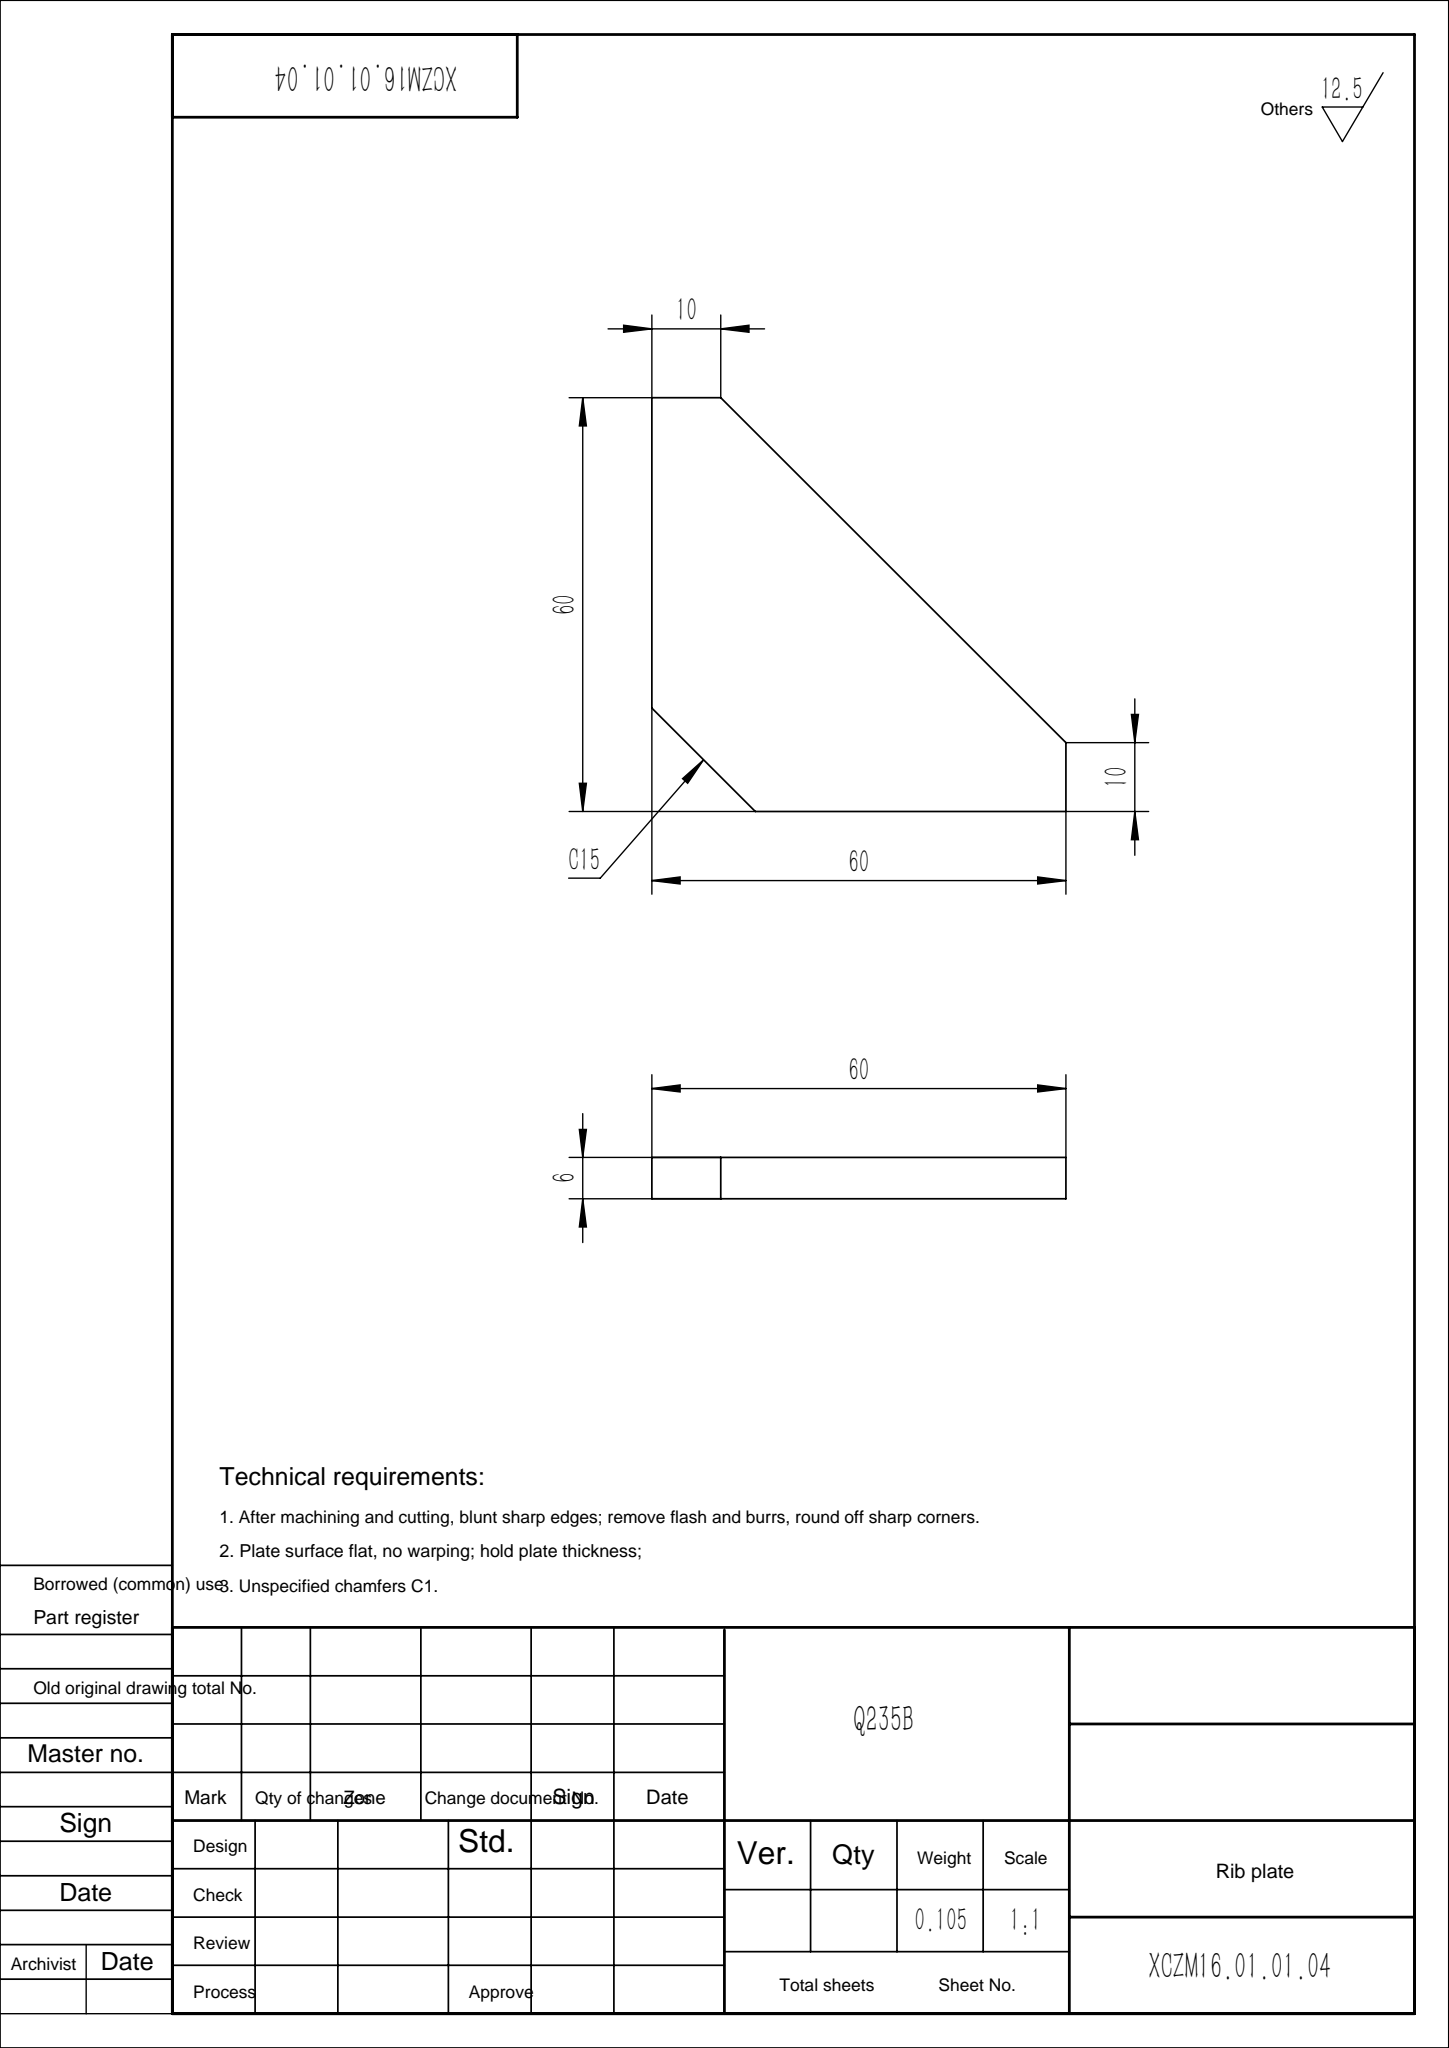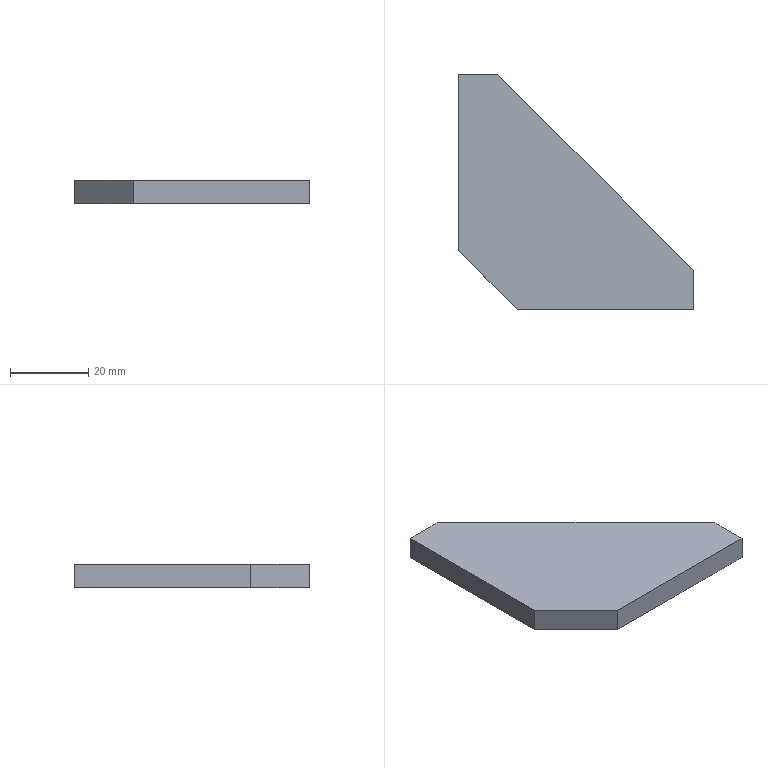Part | SolidWorks | features Chamfer 1, Extrusion 1 | 1 solid | 8 faces | box 60 x 60 x 6 mm | volume 13425 mm3 | plane 8
STEP:
#1=CARTESIAN_POINT('',(10.,60.,0.));
#2=VERTEX_POINT('',#1);
#3=CARTESIAN_POINT('',(0.,60.,0.));
#4=VERTEX_POINT('',#3);
#5=CARTESIAN_POINT('',(10.,60.,0.));
#6=DIRECTION('',(-1.,0.,0.));
#7=VECTOR('',#6,1000.);
#8=LINE('',#5,#7);
#9=EDGE_CURVE('',#2,#4,#8,.T.);
#10=ORIENTED_EDGE('',*,*,#9,.T.);
#11=CARTESIAN_POINT('',(0.,60.,6.));
#12=VERTEX_POINT('',#11);
#13=CARTESIAN_POINT('',(0.,60.,6.));
#14=DIRECTION('',(0.,0.,-1.));
#15=VECTOR('',#14,1000.);
#16=LINE('',#13,#15);
#17=EDGE_CURVE('',#12,#4,#16,.T.);
#18=ORIENTED_EDGE('',*,*,#17,.F.);
#19=CARTESIAN_POINT('',(10.,60.,6.));
#20=VERTEX_POINT('',#19);
#21=CARTESIAN_POINT('',(10.,60.,6.));
#22=DIRECTION('',(-1.,0.,0.));
#23=VECTOR('',#22,1000.);
#24=LINE('',#21,#23);
#25=EDGE_CURVE('',#20,#12,#24,.T.);
#26=ORIENTED_EDGE('',*,*,#25,.F.);
#27=CARTESIAN_POINT('',(10.,60.,6.));
#28=DIRECTION('',(0.,0.,-1.));
#29=VECTOR('',#28,1000.);
#30=LINE('',#27,#29);
#31=EDGE_CURVE('',#20,#2,#30,.T.);
#32=ORIENTED_EDGE('',*,*,#31,.T.);
#33=EDGE_LOOP('',(#10,#18,#26,#32));
#34=FACE_OUTER_BOUND('',#33,.T.);
#35=CARTESIAN_POINT('',(10.,60.,6.));
#36=DIRECTION('',(0.,-1.,0.));
#37=DIRECTION('',(0.,0.,-1.));
#38=AXIS2_PLACEMENT_3D('',#35,#36,#37);
#39=PLANE('',#38);
#40=ADVANCED_FACE('',(#34),#39,.F.);
#41=CARTESIAN_POINT('',(0.,15.,0.));
#42=VERTEX_POINT('',#41);
#43=CARTESIAN_POINT('',(0.,60.,0.));
#44=DIRECTION('',(0.,-1.,0.));
#45=VECTOR('',#44,1000.);
#46=LINE('',#43,#45);
#47=EDGE_CURVE('',#4,#42,#46,.T.);
#48=ORIENTED_EDGE('',*,*,#47,.T.);
#49=CARTESIAN_POINT('',(0.,15.,6.));
#50=VERTEX_POINT('',#49);
#51=CARTESIAN_POINT('',(0.,15.,6.));
#52=DIRECTION('',(0.,0.,1.));
#53=VECTOR('',#52,1000.);
#54=LINE('',#51,#53);
#55=EDGE_CURVE('',#42,#50,#54,.T.);
#56=ORIENTED_EDGE('',*,*,#55,.T.);
#57=CARTESIAN_POINT('',(0.,60.,6.));
#58=DIRECTION('',(0.,-1.,0.));
#59=VECTOR('',#58,1000.);
#60=LINE('',#57,#59);
#61=EDGE_CURVE('',#12,#50,#60,.T.);
#62=ORIENTED_EDGE('',*,*,#61,.F.);
#63=ORIENTED_EDGE('',*,*,#17,.T.);
#64=EDGE_LOOP('',(#48,#56,#62,#63));
#65=FACE_OUTER_BOUND('',#64,.T.);
#66=CARTESIAN_POINT('',(0.,60.,6.));
#67=DIRECTION('',(1.,0.,0.));
#68=DIRECTION('',(0.,1.,0.));
#69=AXIS2_PLACEMENT_3D('',#66,#67,#68);
#70=PLANE('',#69);
#71=ADVANCED_FACE('',(#65),#70,.F.);
#72=CARTESIAN_POINT('',(15.,0.,6.));
#73=VERTEX_POINT('',#72);
#74=CARTESIAN_POINT('',(60.,0.,6.));
#75=VERTEX_POINT('',#74);
#76=CARTESIAN_POINT('',(0.,0.,6.));
#77=DIRECTION('',(1.,0.,0.));
#78=VECTOR('',#77,1000.);
#79=LINE('',#76,#78);
#80=EDGE_CURVE('',#73,#75,#79,.T.);
#81=ORIENTED_EDGE('',*,*,#80,.F.);
#82=CARTESIAN_POINT('',(15.,0.,0.));
#83=VERTEX_POINT('',#82);
#84=CARTESIAN_POINT('',(15.,0.,6.));
#85=DIRECTION('',(0.,0.,-1.));
#86=VECTOR('',#85,1000.);
#87=LINE('',#84,#86);
#88=EDGE_CURVE('',#73,#83,#87,.T.);
#89=ORIENTED_EDGE('',*,*,#88,.T.);
#90=CARTESIAN_POINT('',(60.,0.,0.));
#91=VERTEX_POINT('',#90);
#92=CARTESIAN_POINT('',(0.,0.,0.));
#93=DIRECTION('',(1.,0.,0.));
#94=VECTOR('',#93,1000.);
#95=LINE('',#92,#94);
#96=EDGE_CURVE('',#83,#91,#95,.T.);
#97=ORIENTED_EDGE('',*,*,#96,.T.);
#98=CARTESIAN_POINT('',(60.,0.,6.));
#99=DIRECTION('',(0.,0.,-1.));
#100=VECTOR('',#99,1000.);
#101=LINE('',#98,#100);
#102=EDGE_CURVE('',#75,#91,#101,.T.);
#103=ORIENTED_EDGE('',*,*,#102,.F.);
#104=EDGE_LOOP('',(#81,#89,#97,#103));
#105=FACE_OUTER_BOUND('',#104,.T.);
#106=CARTESIAN_POINT('',(0.,0.,6.));
#107=DIRECTION('',(0.,1.,0.));
#108=DIRECTION('',(0.,0.,1.));
#109=AXIS2_PLACEMENT_3D('',#106,#107,#108);
#110=PLANE('',#109);
#111=ADVANCED_FACE('',(#105),#110,.F.);
#112=CARTESIAN_POINT('',(60.,10.,0.));
#113=VERTEX_POINT('',#112);
#114=CARTESIAN_POINT('',(60.,0.,0.));
#115=DIRECTION('',(0.,1.,0.));
#116=VECTOR('',#115,1000.);
#117=LINE('',#114,#116);
#118=EDGE_CURVE('',#91,#113,#117,.T.);
#119=ORIENTED_EDGE('',*,*,#118,.T.);
#120=CARTESIAN_POINT('',(60.,10.,6.));
#121=VERTEX_POINT('',#120);
#122=CARTESIAN_POINT('',(60.,10.,6.));
#123=DIRECTION('',(0.,0.,-1.));
#124=VECTOR('',#123,1000.);
#125=LINE('',#122,#124);
#126=EDGE_CURVE('',#121,#113,#125,.T.);
#127=ORIENTED_EDGE('',*,*,#126,.F.);
#128=CARTESIAN_POINT('',(60.,0.,6.));
#129=DIRECTION('',(0.,1.,0.));
#130=VECTOR('',#129,1000.);
#131=LINE('',#128,#130);
#132=EDGE_CURVE('',#75,#121,#131,.T.);
#133=ORIENTED_EDGE('',*,*,#132,.F.);
#134=ORIENTED_EDGE('',*,*,#102,.T.);
#135=EDGE_LOOP('',(#119,#127,#133,#134));
#136=FACE_OUTER_BOUND('',#135,.T.);
#137=CARTESIAN_POINT('',(60.,0.,6.));
#138=DIRECTION('',(-1.,0.,0.));
#139=DIRECTION('',(0.,0.,1.));
#140=AXIS2_PLACEMENT_3D('',#137,#138,#139);
#141=PLANE('',#140);
#142=ADVANCED_FACE('',(#136),#141,.F.);
#143=CARTESIAN_POINT('',(60.,10.,0.));
#144=DIRECTION('',(-0.7071,0.7071,0.));
#145=VECTOR('',#144,1000.);
#146=LINE('',#143,#145);
#147=EDGE_CURVE('',#113,#2,#146,.T.);
#148=ORIENTED_EDGE('',*,*,#147,.T.);
#149=ORIENTED_EDGE('',*,*,#31,.F.);
#150=CARTESIAN_POINT('',(60.,10.,6.));
#151=DIRECTION('',(-0.7071,0.7071,0.));
#152=VECTOR('',#151,1000.);
#153=LINE('',#150,#152);
#154=EDGE_CURVE('',#121,#20,#153,.T.);
#155=ORIENTED_EDGE('',*,*,#154,.F.);
#156=ORIENTED_EDGE('',*,*,#126,.T.);
#157=EDGE_LOOP('',(#148,#149,#155,#156));
#158=FACE_OUTER_BOUND('',#157,.T.);
#159=CARTESIAN_POINT('',(60.,10.,6.));
#160=DIRECTION('',(-0.7071,-0.7071,0.));
#161=DIRECTION('',(0.7071,-0.7071,0.));
#162=AXIS2_PLACEMENT_3D('',#159,#160,#161);
#163=PLANE('',#162);
#164=ADVANCED_FACE('',(#158),#163,.F.);
#165=ORIENTED_EDGE('',*,*,#61,.T.);
#166=CARTESIAN_POINT('',(7.5,7.5,6.));
#167=DIRECTION('',(0.7071,-0.7071,0.));
#168=VECTOR('',#167,1000.);
#169=LINE('',#166,#168);
#170=EDGE_CURVE('',#50,#73,#169,.T.);
#171=ORIENTED_EDGE('',*,*,#170,.T.);
#172=ORIENTED_EDGE('',*,*,#80,.T.);
#173=ORIENTED_EDGE('',*,*,#132,.T.);
#174=ORIENTED_EDGE('',*,*,#154,.T.);
#175=ORIENTED_EDGE('',*,*,#25,.T.);
#176=EDGE_LOOP('',(#165,#171,#172,#173,#174,#175));
#177=FACE_OUTER_BOUND('',#176,.T.);
#178=CARTESIAN_POINT('',(0.,0.,6.));
#179=DIRECTION('',(0.,0.,1.));
#180=DIRECTION('',(1.,0.,0.));
#181=AXIS2_PLACEMENT_3D('',#178,#179,#180);
#182=PLANE('',#181);
#183=ADVANCED_FACE('',(#177),#182,.T.);
#184=ORIENTED_EDGE('',*,*,#96,.F.);
#185=CARTESIAN_POINT('',(15.,0.,0.));
#186=DIRECTION('',(-0.7071,0.7071,0.));
#187=VECTOR('',#186,1000.);
#188=LINE('',#185,#187);
#189=EDGE_CURVE('',#83,#42,#188,.T.);
#190=ORIENTED_EDGE('',*,*,#189,.T.);
#191=ORIENTED_EDGE('',*,*,#47,.F.);
#192=ORIENTED_EDGE('',*,*,#9,.F.);
#193=ORIENTED_EDGE('',*,*,#147,.F.);
#194=ORIENTED_EDGE('',*,*,#118,.F.);
#195=EDGE_LOOP('',(#184,#190,#191,#192,#193,#194));
#196=FACE_OUTER_BOUND('',#195,.T.);
#197=CARTESIAN_POINT('',(0.,0.,0.));
#198=DIRECTION('',(0.,0.,1.));
#199=DIRECTION('',(1.,0.,0.));
#200=AXIS2_PLACEMENT_3D('',#197,#198,#199);
#201=PLANE('',#200);
#202=ADVANCED_FACE('',(#196),#201,.F.);
#203=ORIENTED_EDGE('',*,*,#170,.F.);
#204=ORIENTED_EDGE('',*,*,#55,.F.);
#205=ORIENTED_EDGE('',*,*,#189,.F.);
#206=ORIENTED_EDGE('',*,*,#88,.F.);
#207=EDGE_LOOP('',(#203,#204,#205,#206));
#208=FACE_OUTER_BOUND('',#207,.T.);
#209=CARTESIAN_POINT('',(15.,0.,6.));
#210=DIRECTION('',(0.7071,0.7071,0.));
#211=DIRECTION('',(0.,0.,-1.));
#212=AXIS2_PLACEMENT_3D('',#209,#210,#211);
#213=PLANE('',#212);
#214=ADVANCED_FACE('',(#208),#213,.F.);
#215=CLOSED_SHELL('',(#40,#71,#111,#142,#164,#183,#202,#214));
#216=MANIFOLD_SOLID_BREP('',#215);
#217=CARTESIAN_POINT('',(0.,0.,0.));
#218=DIRECTION('',(0.,0.,1.));
#219=DIRECTION('',(1.,0.,0.));
#220=AXIS2_PLACEMENT_3D('',#217,#218,#219);
#221=(LENGTH_UNIT()NAMED_UNIT(*)SI_UNIT(.MILLI.,.METRE.));
#222=UNCERTAINTY_MEASURE_WITH_UNIT(LENGTH_MEASURE(0.00001),#221,'','');
#223=(NAMED_UNIT(*)PLANE_ANGLE_UNIT()SI_UNIT($,.RADIAN.));
#224=(NAMED_UNIT(*)SI_UNIT($,.STERADIAN.)SOLID_ANGLE_UNIT());
#225=(GEOMETRIC_REPRESENTATION_CONTEXT(3)GLOBAL_UNCERTAINTY_ASSIGNED_CONTEXT((#222))GLOBAL_UNIT_ASSIGNED_CONTEXT((#221,#223,#224))REPRESENTATION_CONTEXT('',''));
#226=ADVANCED_BREP_SHAPE_REPRESENTATION('',(#216,#220),#225);